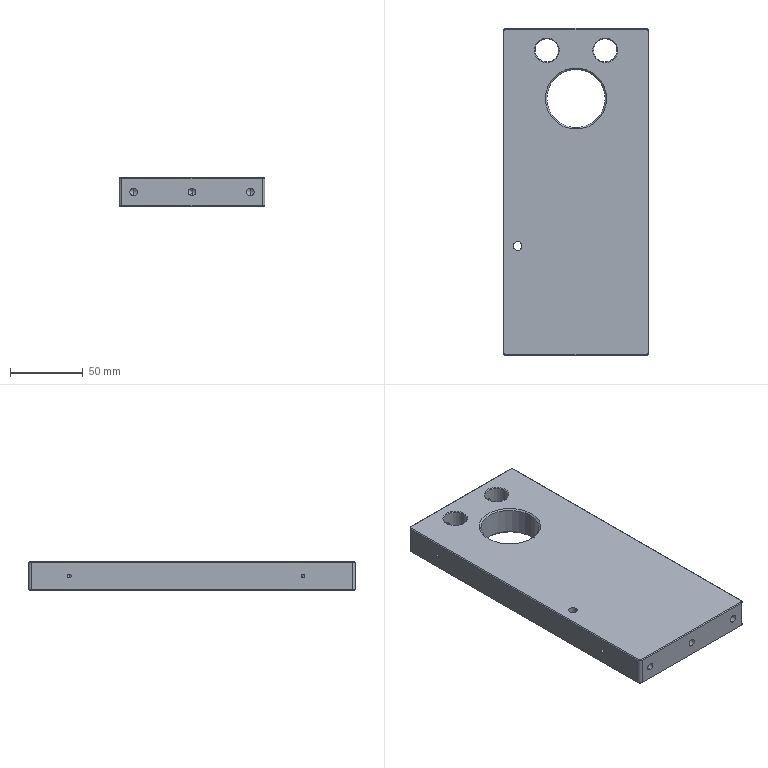Part | STEP file | Guide wheel mechanism revised.sldasm-Part-38 | 1 solid | 70 faces | box 100 x 224 x 19.6 mm | volume 404407 mm3 | cone 30 | cylinder 26 | plane 14 | commonest cylinder face diameters 5 x6 2.5 x4 4 x4 4.2 x4 16 x4 6 x2